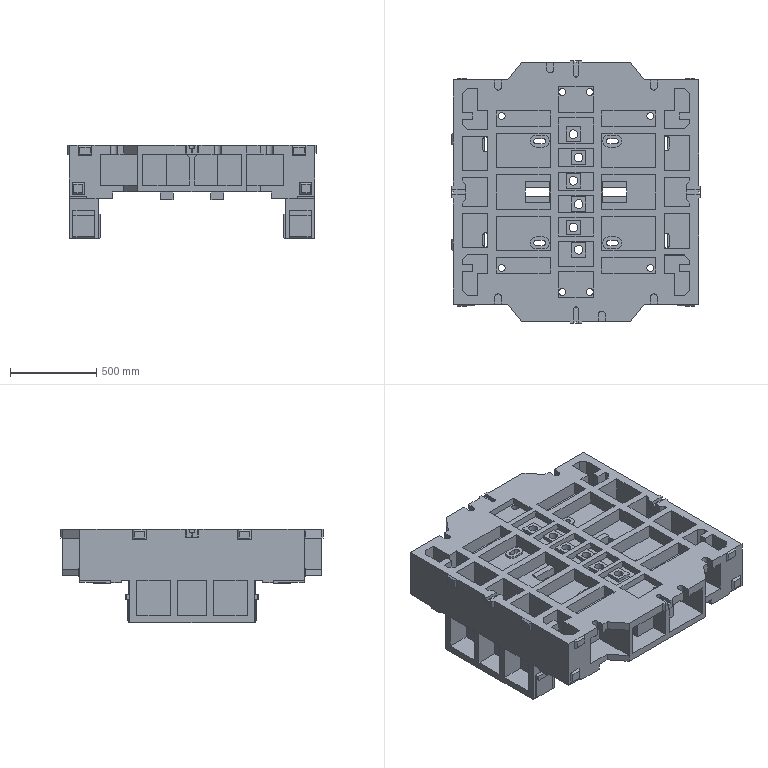Part | NX | features solid 2 | 1 solid | 872 faces | box 1440 x 1520 x 540 mm | volume 272856258 mm3 | plane 780 | cylinder 89 | cone 3 | commonest cylinder face diameters 30 x25 40 x22 20 x10 70 x8 10 x6 51 x6